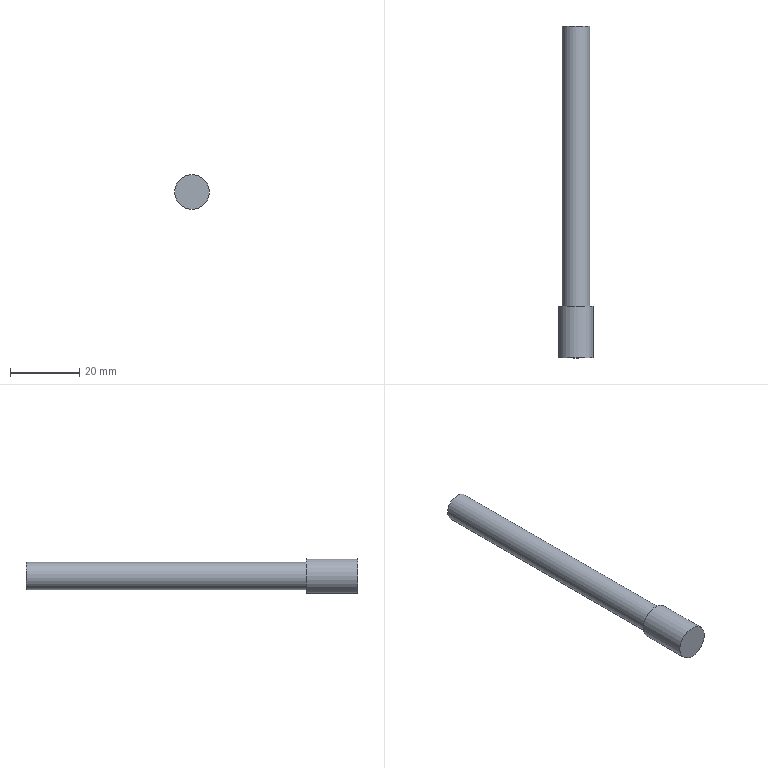Part | STEP file | solid 120 | 1 solid | 5 faces | box 10 x 96 x 10 mm | volume 5250 mm3 | plane 3 | cylinder 2 | commonest cylinder face diameters 8 x1 10 x1